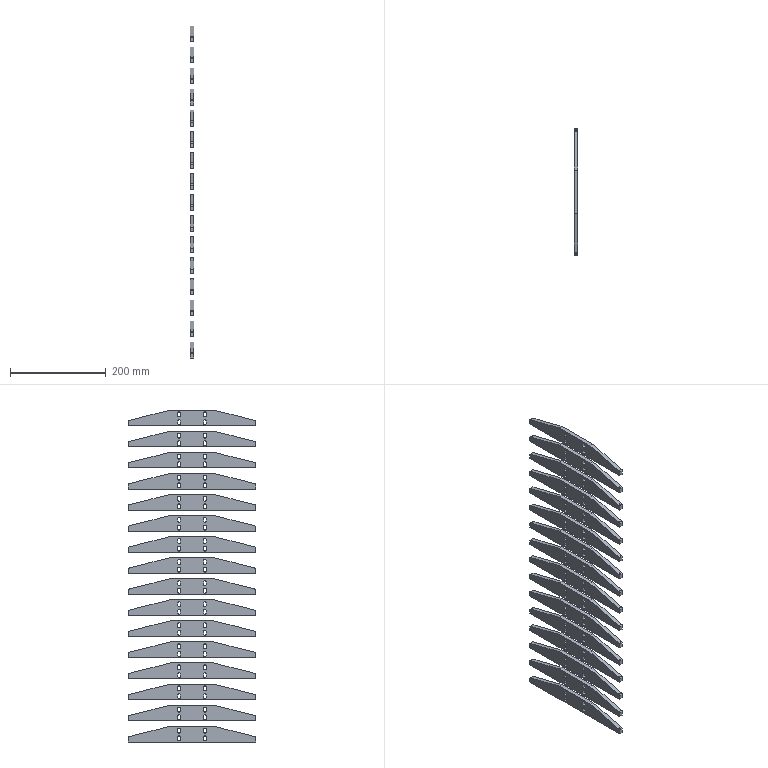CAM job | NX | 3+2 milling | part box 8 x 265.5 x 693 mm | stock box 8 x 270.5 x 698 mm
Tools:
number,name,description,diameter,corner_radius,flute_length,length,flutes
4,D4,平底铣刀-粗,4.0,0.0,25.0,75.0,2
9,D10,平底铣刀-粗,10.0,0.0,35.0,75.0,2
11,D4-J,平底铣刀-精,4.0,0.0,50.0,75.0,2
7,D6-J,平底铣刀-精,6.0,0.0,25.0,75.0,2
2,D6倒角刀,倒角刀,6.0,0.0,3.0,25.0,2
Operations:
program,operation,operation_type,tool,method,geometry_group,spindle_rpm,surface_speed,feed_per_tooth,feed_cut,feed_plunge,cut_length_mm,path_length_mm,cut_time_min,machine_time_min
B,C0.3封闭铣廓倒角6X45L_COPY,PlanarMilling,D6倒角刀,爬面_倒角-切深0-步距G,W-B,7000.0,131.0,0.1071,1500.0,100.0,718.635,1496.253,0.4791,0.5569
A,通腰槽粗_1,VolumeBased25DMillingOperation,D4,METHOD,W-A,6000.0,75.398,0.1,1200.0,100.0,31648.921,36978.814,26.374,26.907
A,外形粗_2,VolumeBased25DMillingOperation,D10,METHOD,W-A,6000.0,188.0,0.25,4000.0,80.0,160194.955,161678.195,40.049,40.197
A,腰槽精_1,VolumeBased25DMillingOperation,D4-J,METHOD,W-A,6000.0,113.0,0.0417,500.0,100.0,2168.411,8649.487,4.337,4.985
A,仅选体,SurfaceContour,D6倒角刀,METHOD,W-A,6000.0,113.0,0.125,1200.0,100.0,10994.384,16940.822,9.162,9.757
A,外形半精_2,VolumeBased25DMillingOperation,D6-J,METHOD,W-A,6000.0,113.0,0.0833,1000.0,100.0,9289.977,11050.344,9.29,9.466
A,外形精_2,VolumeBased25DMillingOperation,D6-J,METHOD,W-A,6000.0,113.0,0.0833,1000.0,100.0,9286.777,11056.634,9.287,9.464